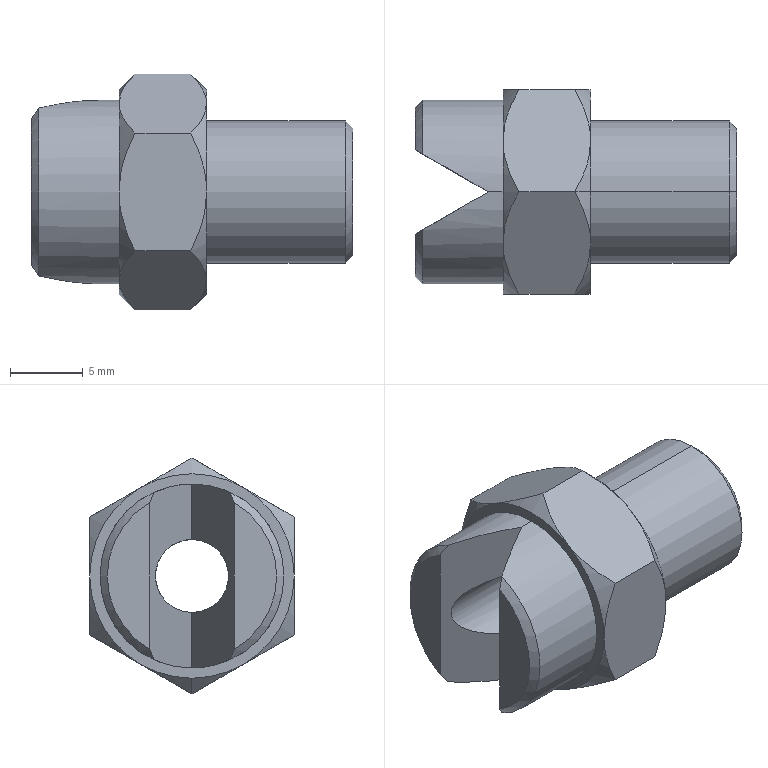Part | SolidWorks | features ICE 3, RevCut 1, Revolution 1 | 1 solid | 40 faces | box 22 x 14 x 16.166 mm | volume 1551 mm3 | cone 18 | plane 14 | cylinder 8 | commonest cylinder face diameters 5 x2 7.5 x2 9.728 x2 12.6 x2
STEP:
#1=CARTESIAN_POINT('',(5.,0.,2.5));
#2=VERTEX_POINT('',#1);
#3=CARTESIAN_POINT('',(5.,0.,-2.5));
#4=VERTEX_POINT('',#3);
#5=CARTESIAN_POINT('',(5.,0.,2.5));
#6=CARTESIAN_POINT('',(-3.66,-5.,2.5));
#7=CARTESIAN_POINT('',(-3.66,-5.,-2.5));
#8=CARTESIAN_POINT('',(5.,0.,-2.5));
#9=(BOUNDED_CURVE()B_SPLINE_CURVE(3,(#5,#6,#7,#8),.UNSPECIFIED.,.F.,.T.)B_SPLINE_CURVE_WITH_KNOTS((4,4),(1.571,4.712),.UNSPECIFIED.)CURVE()GEOMETRIC_REPRESENTATION_ITEM()RATIONAL_B_SPLINE_CURVE((1.,0.3333,0.3333,1.))REPRESENTATION_ITEM(''));
#10=EDGE_CURVE('',#2,#4,#9,.T.);
#11=ORIENTED_EDGE('',*,*,#10,.F.);
#12=CARTESIAN_POINT('',(6.,0.,2.5));
#13=VERTEX_POINT('',#12);
#14=CARTESIAN_POINT('',(0.,0.,2.5));
#15=DIRECTION('',(1.,0.,0.));
#16=VECTOR('',#15,1000.);
#17=LINE('',#14,#16);
#18=EDGE_CURVE('',#2,#13,#17,.T.);
#19=ORIENTED_EDGE('',*,*,#18,.T.);
#20=CARTESIAN_POINT('',(6.,0.,-2.5));
#21=VERTEX_POINT('',#20);
#22=CARTESIAN_POINT('',(6.,0.,0.));
#23=DIRECTION('',(1.,0.,0.));
#24=DIRECTION('',(0.,0.,-1.));
#25=AXIS2_PLACEMENT_3D('',#22,#23,#24);
#26=CIRCLE('',#25,2.5);
#27=EDGE_CURVE('',#13,#21,#26,.T.);
#28=ORIENTED_EDGE('',*,*,#27,.T.);
#29=CARTESIAN_POINT('',(0.,0.,-2.5));
#30=DIRECTION('',(1.,0.,0.));
#31=VECTOR('',#30,1000.);
#32=LINE('',#29,#31);
#33=EDGE_CURVE('',#4,#21,#32,.T.);
#34=ORIENTED_EDGE('',*,*,#33,.F.);
#35=EDGE_LOOP('',(#11,#19,#28,#34));
#36=FACE_OUTER_BOUND('',#35,.T.);
#37=CARTESIAN_POINT('',(0.,0.,0.));
#38=DIRECTION('',(1.,0.,0.));
#39=DIRECTION('',(0.,0.,-1.));
#40=AXIS2_PLACEMENT_3D('',#37,#38,#39);
#41=CYLINDRICAL_SURFACE('',#40,2.5);
#42=ADVANCED_FACE('',(#36),#41,.F.);
#43=CARTESIAN_POINT('',(6.,0.,6.3));
#44=VERTEX_POINT('',#43);
#45=CARTESIAN_POINT('',(6.,0.,-6.3));
#46=VERTEX_POINT('',#45);
#47=CARTESIAN_POINT('',(6.,0.,0.));
#48=DIRECTION('',(-1.,0.,0.));
#49=DIRECTION('',(0.,0.,1.));
#50=AXIS2_PLACEMENT_3D('',#47,#48,#49);
#51=CIRCLE('',#50,6.3);
#52=EDGE_CURVE('',#44,#46,#51,.T.);
#53=ORIENTED_EDGE('',*,*,#52,.T.);
#54=CARTESIAN_POINT('',(5.,0.,-6.3));
#55=VERTEX_POINT('',#54);
#56=CARTESIAN_POINT('',(0.,0.,-6.3));
#57=DIRECTION('',(-1.,0.,0.));
#58=VECTOR('',#57,1000.);
#59=LINE('',#56,#58);
#60=EDGE_CURVE('',#46,#55,#59,.T.);
#61=ORIENTED_EDGE('',*,*,#60,.T.);
#62=CARTESIAN_POINT('',(0.5,2.598,-5.739));
#63=VERTEX_POINT('',#62);
#64=CARTESIAN_POINT('',(5.,0.,-6.3));
#65=CARTESIAN_POINT('',(3.442,0.8995,-6.3));
#66=CARTESIAN_POINT('',(1.919,1.779,-6.11));
#67=CARTESIAN_POINT('',(0.5,2.598,-5.739));
#68=(BOUNDED_CURVE()B_SPLINE_CURVE(3,(#64,#65,#66,#67),.UNSPECIFIED.,.F.,.T.)B_SPLINE_CURVE_WITH_KNOTS((4,4),(4.712,5.137),.UNSPECIFIED.)CURVE()GEOMETRIC_REPRESENTATION_ITEM()RATIONAL_B_SPLINE_CURVE((1.,0.985,0.985,1.))REPRESENTATION_ITEM(''));
#69=EDGE_CURVE('',#55,#63,#68,.T.);
#70=ORIENTED_EDGE('',*,*,#69,.T.);
#71=CARTESIAN_POINT('',(0.5,2.598,5.739));
#72=VERTEX_POINT('',#71);
#73=CARTESIAN_POINT('',(0.5,0.,0.));
#74=DIRECTION('',(-1.,0.,0.));
#75=DIRECTION('',(0.,0.,1.));
#76=AXIS2_PLACEMENT_3D('',#73,#74,#75);
#77=CIRCLE('',#76,6.3);
#78=EDGE_CURVE('',#72,#63,#77,.T.);
#79=ORIENTED_EDGE('',*,*,#78,.F.);
#80=CARTESIAN_POINT('',(5.,0.,6.3));
#81=VERTEX_POINT('',#80);
#82=CARTESIAN_POINT('',(0.5,2.598,5.739));
#83=CARTESIAN_POINT('',(1.919,1.779,6.11));
#84=CARTESIAN_POINT('',(3.442,0.8995,6.3));
#85=CARTESIAN_POINT('',(5.,0.,6.3));
#86=(BOUNDED_CURVE()B_SPLINE_CURVE(3,(#82,#83,#84,#85),.UNSPECIFIED.,.F.,.F.)B_SPLINE_CURVE_WITH_KNOTS((4,4),(1.146,1.571),.UNSPECIFIED.)CURVE()GEOMETRIC_REPRESENTATION_ITEM()RATIONAL_B_SPLINE_CURVE((1.,0.985,0.985,1.))REPRESENTATION_ITEM(''));
#87=EDGE_CURVE('',#72,#81,#86,.T.);
#88=ORIENTED_EDGE('',*,*,#87,.T.);
#89=CARTESIAN_POINT('',(0.,0.,6.3));
#90=DIRECTION('',(-1.,0.,0.));
#91=VECTOR('',#90,1000.);
#92=LINE('',#89,#91);
#93=EDGE_CURVE('',#44,#81,#92,.T.);
#94=ORIENTED_EDGE('',*,*,#93,.F.);
#95=EDGE_LOOP('',(#53,#61,#70,#79,#88,#94));
#96=FACE_OUTER_BOUND('',#95,.T.);
#97=CARTESIAN_POINT('',(0.,0.,0.));
#98=DIRECTION('',(-1.,0.,0.));
#99=DIRECTION('',(0.,0.,1.));
#100=AXIS2_PLACEMENT_3D('',#97,#98,#99);
#101=CYLINDRICAL_SURFACE('',#100,6.3);
#102=ADVANCED_FACE('',(#96),#101,.T.);
#103=CARTESIAN_POINT('',(6.,-3.5,-6.062));
#104=VERTEX_POINT('',#103);
#105=CARTESIAN_POINT('',(6.,0.,-7.));
#106=VERTEX_POINT('',#105);
#107=CARTESIAN_POINT('',(6.,0.,0.));
#108=DIRECTION('',(1.,0.,0.));
#109=DIRECTION('',(0.,0.,-1.));
#110=AXIS2_PLACEMENT_3D('',#107,#108,#109);
#111=CIRCLE('',#110,7.);
#112=EDGE_CURVE('',#104,#106,#111,.T.);
#113=ORIENTED_EDGE('',*,*,#112,.T.);
#114=CARTESIAN_POINT('',(7.083,0.,-8.083));
#115=VERTEX_POINT('',#114);
#116=CARTESIAN_POINT('',(6.,0.,-7.));
#117=DIRECTION('',(0.7071,0.,-0.7071));
#118=VECTOR('',#117,1000.);
#119=LINE('',#116,#118);
#120=EDGE_CURVE('',#106,#115,#119,.T.);
#121=ORIENTED_EDGE('',*,*,#120,.T.);
#122=CARTESIAN_POINT('',(7.083,0.,-8.083));
#123=CARTESIAN_POINT('',(6.766,-0.5488,-7.766));
#124=CARTESIAN_POINT('',(6.497,-1.11,-7.442));
#125=CARTESIAN_POINT('',(6.209,-1.982,-6.938));
#126=CARTESIAN_POINT('',(6.132,-2.278,-6.768));
#127=CARTESIAN_POINT('',(6.028,-2.882,-6.419));
#128=CARTESIAN_POINT('',(6.,-3.193,-6.239));
#129=CARTESIAN_POINT('',(6.,-3.5,-6.062));
#130=B_SPLINE_CURVE_WITH_KNOTS('',3,(#122,#123,#124,#125,#126,#127,#128,#129),.UNSPECIFIED.,.F.,.F.,(4,2,2,4),(0.000000254,0.002095,0.003142,0.00419),.UNSPECIFIED.);
#131=EDGE_CURVE('',#115,#104,#130,.T.);
#132=ORIENTED_EDGE('',*,*,#131,.T.);
#133=EDGE_LOOP('',(#113,#121,#132));
#134=FACE_OUTER_BOUND('',#133,.T.);
#135=CARTESIAN_POINT('',(6.,0.,0.));
#136=DIRECTION('',(1.,0.,0.));
#137=DIRECTION('',(0.,0.,-1.));
#138=AXIS2_PLACEMENT_3D('',#135,#136,#137);
#139=CONICAL_SURFACE('',#138,7.,0.7854);
#140=ADVANCED_FACE('',(#134),#139,.T.);
#141=CARTESIAN_POINT('',(12.,0.,7.));
#142=VERTEX_POINT('',#141);
#143=CARTESIAN_POINT('',(12.,-3.5,6.062));
#144=VERTEX_POINT('',#143);
#145=CARTESIAN_POINT('',(12.,0.,0.));
#146=DIRECTION('',(1.,0.,0.));
#147=DIRECTION('',(0.,0.,-1.));
#148=AXIS2_PLACEMENT_3D('',#145,#146,#147);
#149=CIRCLE('',#148,7.);
#150=EDGE_CURVE('',#142,#144,#149,.T.);
#151=ORIENTED_EDGE('',*,*,#150,.F.);
#152=CARTESIAN_POINT('',(10.917,0.,8.083));
#153=VERTEX_POINT('',#152);
#154=CARTESIAN_POINT('',(10.917,0.,8.083));
#155=DIRECTION('',(-0.7071,0.,0.7071));
#156=VECTOR('',#155,1000.);
#157=LINE('',#154,#156);
#158=EDGE_CURVE('',#142,#153,#157,.T.);
#159=ORIENTED_EDGE('',*,*,#158,.T.);
#160=CARTESIAN_POINT('',(10.917,0.,8.083));
#161=CARTESIAN_POINT('',(11.234,-0.5488,7.766));
#162=CARTESIAN_POINT('',(11.503,-1.11,7.442));
#163=CARTESIAN_POINT('',(11.791,-1.982,6.938));
#164=CARTESIAN_POINT('',(11.868,-2.278,6.768));
#165=CARTESIAN_POINT('',(11.972,-2.882,6.419));
#166=CARTESIAN_POINT('',(12.,-3.193,6.239));
#167=CARTESIAN_POINT('',(12.,-3.5,6.062));
#168=B_SPLINE_CURVE_WITH_KNOTS('',3,(#160,#161,#162,#163,#164,#165,#166,#167),.UNSPECIFIED.,.F.,.F.,(4,2,2,4),(0.000000254,0.002095,0.003142,0.00419),.UNSPECIFIED.);
#169=EDGE_CURVE('',#153,#144,#168,.T.);
#170=ORIENTED_EDGE('',*,*,#169,.T.);
#171=EDGE_LOOP('',(#151,#159,#170));
#172=FACE_OUTER_BOUND('',#171,.T.);
#173=CARTESIAN_POINT('',(10.917,0.,0.));
#174=DIRECTION('',(-1.,0.,0.));
#175=DIRECTION('',(0.,0.,1.));
#176=AXIS2_PLACEMENT_3D('',#173,#174,#175);
#177=CONICAL_SURFACE('',#176,8.083,0.7854);
#178=ADVANCED_FACE('',(#172),#177,.T.);
#179=CARTESIAN_POINT('',(22.,0.,-3.75));
#180=VERTEX_POINT('',#179);
#181=CARTESIAN_POINT('',(22.,0.,3.75));
#182=VERTEX_POINT('',#181);
#183=CARTESIAN_POINT('',(22.,0.,0.));
#184=DIRECTION('',(-1.,0.,0.));
#185=DIRECTION('',(0.,0.,1.));
#186=AXIS2_PLACEMENT_3D('',#183,#184,#185);
#187=CIRCLE('',#186,3.75);
#188=EDGE_CURVE('',#180,#182,#187,.T.);
#189=ORIENTED_EDGE('',*,*,#188,.F.);
#190=CARTESIAN_POINT('',(6.,0.,-3.75));
#191=VERTEX_POINT('',#190);
#192=CARTESIAN_POINT('',(0.,0.,-3.75));
#193=DIRECTION('',(-1.,0.,0.));
#194=VECTOR('',#193,1000.);
#195=LINE('',#192,#194);
#196=EDGE_CURVE('',#180,#191,#195,.T.);
#197=ORIENTED_EDGE('',*,*,#196,.T.);
#198=CARTESIAN_POINT('',(6.,0.,3.75));
#199=VERTEX_POINT('',#198);
#200=CARTESIAN_POINT('',(6.,0.,0.));
#201=DIRECTION('',(-1.,0.,0.));
#202=DIRECTION('',(0.,0.,1.));
#203=AXIS2_PLACEMENT_3D('',#200,#201,#202);
#204=CIRCLE('',#203,3.75);
#205=EDGE_CURVE('',#191,#199,#204,.T.);
#206=ORIENTED_EDGE('',*,*,#205,.T.);
#207=CARTESIAN_POINT('',(0.,0.,3.75));
#208=DIRECTION('',(-1.,0.,0.));
#209=VECTOR('',#208,1000.);
#210=LINE('',#207,#209);
#211=EDGE_CURVE('',#182,#199,#210,.T.);
#212=ORIENTED_EDGE('',*,*,#211,.F.);
#213=EDGE_LOOP('',(#189,#197,#206,#212));
#214=FACE_OUTER_BOUND('',#213,.T.);
#215=CARTESIAN_POINT('',(0.,0.,0.));
#216=DIRECTION('',(-1.,0.,0.));
#217=DIRECTION('',(0.,0.,1.));
#218=AXIS2_PLACEMENT_3D('',#215,#216,#217);
#219=CYLINDRICAL_SURFACE('',#218,3.75);
#220=ADVANCED_FACE('',(#214),#219,.F.);
#221=CARTESIAN_POINT('',(22.,0.,4.364));
#222=VERTEX_POINT('',#221);
#223=CARTESIAN_POINT('',(22.,0.,-4.364));
#224=VERTEX_POINT('',#223);
#225=CARTESIAN_POINT('',(22.,0.,0.));
#226=DIRECTION('',(-1.,0.,0.));
#227=DIRECTION('',(0.,0.,1.));
#228=AXIS2_PLACEMENT_3D('',#225,#226,#227);
#229=CIRCLE('',#228,4.364);
#230=EDGE_CURVE('',#222,#224,#229,.T.);
#231=ORIENTED_EDGE('',*,*,#230,.T.);
#232=CARTESIAN_POINT('',(21.5,0.,-4.864));
#233=VERTEX_POINT('',#232);
#234=CARTESIAN_POINT('',(22.,0.,-4.364));
#235=DIRECTION('',(-0.7071,0.,-0.7071));
#236=VECTOR('',#235,1000.);
#237=LINE('',#234,#236);
#238=EDGE_CURVE('',#224,#233,#237,.T.);
#239=ORIENTED_EDGE('',*,*,#238,.T.);
#240=CARTESIAN_POINT('',(21.5,0.,4.864));
#241=VERTEX_POINT('',#240);
#242=CARTESIAN_POINT('',(21.5,0.,0.));
#243=DIRECTION('',(-1.,0.,0.));
#244=DIRECTION('',(0.,0.,1.));
#245=AXIS2_PLACEMENT_3D('',#242,#243,#244);
#246=CIRCLE('',#245,4.864);
#247=EDGE_CURVE('',#241,#233,#246,.T.);
#248=ORIENTED_EDGE('',*,*,#247,.F.);
#249=CARTESIAN_POINT('',(22.,0.,4.364));
#250=DIRECTION('',(-0.7071,0.,0.7071));
#251=VECTOR('',#250,1000.);
#252=LINE('',#249,#251);
#253=EDGE_CURVE('',#222,#241,#252,.T.);
#254=ORIENTED_EDGE('',*,*,#253,.F.);
#255=EDGE_LOOP('',(#231,#239,#248,#254));
#256=FACE_OUTER_BOUND('',#255,.T.);
#257=CARTESIAN_POINT('',(22.,0.,0.));
#258=DIRECTION('',(-1.,0.,0.));
#259=DIRECTION('',(0.,0.,1.));
#260=AXIS2_PLACEMENT_3D('',#257,#258,#259);
#261=CONICAL_SURFACE('',#260,4.364,0.7854);
#262=ADVANCED_FACE('',(#256),#261,.T.);
#263=ORIENTED_EDGE('',*,*,#247,.T.);
#264=CARTESIAN_POINT('',(12.,0.,-4.864));
#265=VERTEX_POINT('',#264);
#266=CARTESIAN_POINT('',(0.,0.,-4.864));
#267=DIRECTION('',(-1.,0.,0.));
#268=VECTOR('',#267,1000.);
#269=LINE('',#266,#268);
#270=EDGE_CURVE('',#233,#265,#269,.T.);
#271=ORIENTED_EDGE('',*,*,#270,.T.);
#272=CARTESIAN_POINT('',(12.,0.,4.864));
#273=VERTEX_POINT('',#272);
#274=CARTESIAN_POINT('',(12.,0.,0.));
#275=DIRECTION('',(-1.,0.,0.));
#276=DIRECTION('',(0.,0.,1.));
#277=AXIS2_PLACEMENT_3D('',#274,#275,#276);
#278=CIRCLE('',#277,4.864);
#279=EDGE_CURVE('',#273,#265,#278,.T.);
#280=ORIENTED_EDGE('',*,*,#279,.F.);
#281=CARTESIAN_POINT('',(0.,0.,4.864));
#282=DIRECTION('',(-1.,0.,0.));
#283=VECTOR('',#282,1000.);
#284=LINE('',#281,#283);
#285=EDGE_CURVE('',#241,#273,#284,.T.);
#286=ORIENTED_EDGE('',*,*,#285,.F.);
#287=EDGE_LOOP('',(#263,#271,#280,#286));
#288=FACE_OUTER_BOUND('',#287,.T.);
#289=CARTESIAN_POINT('',(0.,0.,0.));
#290=DIRECTION('',(-1.,0.,0.));
#291=DIRECTION('',(0.,0.,1.));
#292=AXIS2_PLACEMENT_3D('',#289,#290,#291);
#293=CYLINDRICAL_SURFACE('',#292,4.864);
#294=ADVANCED_FACE('',(#288),#293,.T.);
#295=CARTESIAN_POINT('',(0.,2.887,5.031));
#296=VERTEX_POINT('',#295);
#297=CARTESIAN_POINT('',(0.,2.887,-5.031));
#298=VERTEX_POINT('',#297);
#299=CARTESIAN_POINT('',(0.,0.,0.));
#300=DIRECTION('',(-1.,0.,0.));
#301=DIRECTION('',(0.,0.,1.));
#302=AXIS2_PLACEMENT_3D('',#299,#300,#301);
#303=CIRCLE('',#302,5.8);
#304=EDGE_CURVE('',#296,#298,#303,.T.);
#305=ORIENTED_EDGE('',*,*,#304,.T.);
#306=CARTESIAN_POINT('',(0.,2.887,-8.083));
#307=DIRECTION('',(0.,0.,1.));
#308=VECTOR('',#307,1000.);
#309=LINE('',#306,#308);
#310=EDGE_CURVE('',#298,#296,#309,.T.);
#311=ORIENTED_EDGE('',*,*,#310,.T.);
#312=EDGE_LOOP('',(#305,#311));
#313=FACE_OUTER_BOUND('',#312,.T.);
#314=CARTESIAN_POINT('',(0.,0.,0.));
#315=DIRECTION('',(1.,0.,0.));
#316=DIRECTION('',(0.,0.,-1.));
#317=AXIS2_PLACEMENT_3D('',#314,#315,#316);
#318=PLANE('',#317);
#319=ADVANCED_FACE('',(#313),#318,.F.);
#320=ORIENTED_EDGE('',*,*,#78,.T.);
#321=CARTESIAN_POINT('',(0.5,2.598,-5.739));
#322=CARTESIAN_POINT('',(0.3291,2.697,-5.507));
#323=CARTESIAN_POINT('',(0.1621,2.793,-5.271));
#324=CARTESIAN_POINT('',(0.,2.887,-5.031));
#325=B_SPLINE_CURVE_WITH_KNOTS('',3,(#321,#322,#323,#324),.UNSPECIFIED.,.F.,.F.,(4,4),(0.000000357,0.0009145),.UNSPECIFIED.);
#326=EDGE_CURVE('',#63,#298,#325,.T.);
#327=ORIENTED_EDGE('',*,*,#326,.T.);
#328=ORIENTED_EDGE('',*,*,#304,.F.);
#329=CARTESIAN_POINT('',(0.,2.887,5.031));
#330=CARTESIAN_POINT('',(0.1621,2.793,5.271));
#331=CARTESIAN_POINT('',(0.3291,2.697,5.507));
#332=CARTESIAN_POINT('',(0.5,2.598,5.739));
#333=B_SPLINE_CURVE_WITH_KNOTS('',3,(#329,#330,#331,#332),.UNSPECIFIED.,.F.,.F.,(4,4),(0.000000376,0.0009145),.UNSPECIFIED.);
#334=EDGE_CURVE('',#296,#72,#333,.T.);
#335=ORIENTED_EDGE('',*,*,#334,.T.);
#336=EDGE_LOOP('',(#320,#327,#328,#335));
#337=FACE_OUTER_BOUND('',#336,.T.);
#338=CARTESIAN_POINT('',(0.5,0.,0.));
#339=DIRECTION('',(1.,0.,0.));
#340=DIRECTION('',(0.,0.,-1.));
#341=AXIS2_PLACEMENT_3D('',#338,#339,#340);
#342=CONICAL_SURFACE('',#341,6.3,0.7854);
#343=ADVANCED_FACE('',(#337),#342,.T.);
#344=CARTESIAN_POINT('',(12.,3.5,6.062));
#345=VERTEX_POINT('',#344);
#346=CARTESIAN_POINT('',(12.,0.,0.));
#347=DIRECTION('',(1.,0.,0.));
#348=DIRECTION('',(0.,0.,-1.));
#349=AXIS2_PLACEMENT_3D('',#346,#347,#348);
#350=CIRCLE('',#349,7.);
#351=EDGE_CURVE('',#345,#142,#350,.T.);
#352=ORIENTED_EDGE('',*,*,#351,.T.);
#353=ORIENTED_EDGE('',*,*,#150,.T.);
#354=CARTESIAN_POINT('',(12.,-7.,0.));
#355=VERTEX_POINT('',#354);
#356=CARTESIAN_POINT('',(12.,0.,0.));
#357=DIRECTION('',(1.,0.,0.));
#358=DIRECTION('',(0.,0.,-1.));
#359=AXIS2_PLACEMENT_3D('',#356,#357,#358);
#360=CIRCLE('',#359,7.);
#361=EDGE_CURVE('',#144,#355,#360,.T.);
#362=ORIENTED_EDGE('',*,*,#361,.T.);
#363=CARTESIAN_POINT('',(12.,-3.5,-6.062));
#364=VERTEX_POINT('',#363);
#365=CARTESIAN_POINT('',(12.,0.,0.));
#366=DIRECTION('',(1.,0.,0.));
#367=DIRECTION('',(0.,0.,-1.));
#368=AXIS2_PLACEMENT_3D('',#365,#366,#367);
#369=CIRCLE('',#368,7.);
#370=EDGE_CURVE('',#355,#364,#369,.T.);
#371=ORIENTED_EDGE('',*,*,#370,.T.);
#372=CARTESIAN_POINT('',(12.,3.5,-6.062));
#373=VERTEX_POINT('',#372);
#374=CARTESIAN_POINT('',(12.,0.,0.));
#375=DIRECTION('',(1.,0.,0.));
#376=DIRECTION('',(0.,0.,-1.));
#377=AXIS2_PLACEMENT_3D('',#374,#375,#376);
#378=CIRCLE('',#377,7.);
#379=EDGE_CURVE('',#364,#373,#378,.T.);
#380=ORIENTED_EDGE('',*,*,#379,.T.);
#381=CARTESIAN_POINT('',(12.,7.,0.));
#382=VERTEX_POINT('',#381);
#383=CARTESIAN_POINT('',(12.,0.,0.));
#384=DIRECTION('',(1.,0.,0.));
#385=DIRECTION('',(0.,0.,-1.));
#386=AXIS2_PLACEMENT_3D('',#383,#384,#385);
#387=CIRCLE('',#386,7.);
#388=EDGE_CURVE('',#373,#382,#387,.T.);
#389=ORIENTED_EDGE('',*,*,#388,.T.);
#390=CARTESIAN_POINT('',(12.,0.,0.));
#391=DIRECTION('',(1.,0.,0.));
#392=DIRECTION('',(0.,0.,-1.));
#393=AXIS2_PLACEMENT_3D('',#390,#391,#392);
#394=CIRCLE('',#393,7.);
#395=EDGE_CURVE('',#382,#345,#394,.T.);
#396=ORIENTED_EDGE('',*,*,#395,.T.);
#397=EDGE_LOOP('',(#352,#353,#362,#371,#380,#389,#396));
#398=FACE_OUTER_BOUND('',#397,.T.);
#399=ORIENTED_EDGE('',*,*,#279,.T.);
#400=CARTESIAN_POINT('',(12.,0.,0.));
#401=DIRECTION('',(-1.,0.,0.));
#402=DIRECTION('',(0.,0.,1.));
#403=AXIS2_PLACEMENT_3D('',#400,#401,#402);
#404=CIRCLE('',#403,4.864);
#405=EDGE_CURVE('',#265,#273,#404,.T.);
#406=ORIENTED_EDGE('',*,*,#405,.T.);
#407=EDGE_LOOP('',(#399,#406));
#408=FACE_BOUND('',#407,.T.);
#409=CARTESIAN_POINT('',(12.,7.,0.));
#410=DIRECTION('',(-1.,0.,0.));
#411=DIRECTION('',(0.,0.,1.));
#412=AXIS2_PLACEMENT_3D('',#409,#410,#411);
#413=PLANE('',#412);
#414=ADVANCED_FACE('',(#398,#408),#413,.F.);
#415=ORIENTED_EDGE('',*,*,#270,.F.);
#416=CARTESIAN_POINT('',(21.5,0.,0.));
#417=DIRECTION('',(-1.,0.,0.));
#418=DIRECTION('',(0.,0.,1.));
#419=AXIS2_PLACEMENT_3D('',#416,#417,#418);
#420=CIRCLE('',#419,4.864);
#421=EDGE_CURVE('',#233,#241,#420,.T.);
#422=ORIENTED_EDGE('',*,*,#421,.T.);
#423=ORIENTED_EDGE('',*,*,#285,.T.);
#424=ORIENTED_EDGE('',*,*,#405,.F.);
#425=EDGE_LOOP('',(#415,#422,#423,#424));
#426=FACE_OUTER_BOUND('',#425,.T.);
#427=CARTESIAN_POINT('',(0.,0.,0.));
#428=DIRECTION('',(-1.,0.,0.));
#429=DIRECTION('',(0.,0.,1.));
#430=AXIS2_PLACEMENT_3D('',#427,#428,#429);
#431=CYLINDRICAL_SURFACE('',#430,4.864);
#432=ADVANCED_FACE('',(#426),#431,.T.);
#433=ORIENTED_EDGE('',*,*,#238,.F.);
#434=CARTESIAN_POINT('',(22.,0.,0.));
#435=DIRECTION('',(-1.,0.,0.));
#436=DIRECTION('',(0.,0.,1.));
#437=AXIS2_PLACEMENT_3D('',#434,#435,#436);
#438=CIRCLE('',#437,4.364);
#439=EDGE_CURVE('',#224,#222,#438,.T.);
#440=ORIENTED_EDGE('',*,*,#439,.T.);
#441=ORIENTED_EDGE('',*,*,#253,.T.);
#442=ORIENTED_EDGE('',*,*,#421,.F.);
#443=EDGE_LOOP('',(#433,#440,#441,#442));
#444=FACE_OUTER_BOUND('',#443,.T.);
#445=CARTESIAN_POINT('',(22.,0.,0.));
#446=DIRECTION('',(-1.,0.,0.));
#447=DIRECTION('',(0.,0.,1.));
#448=AXIS2_PLACEMENT_3D('',#445,#446,#447);
#449=CONICAL_SURFACE('',#448,4.364,0.7854);
#450=ADVANCED_FACE('',(#444),#449,.T.);
#451=ORIENTED_EDGE('',*,*,#230,.F.);
#452=ORIENTED_EDGE('',*,*,#439,.F.);
#453=EDGE_LOOP('',(#451,#452));
#454=FACE_OUTER_BOUND('',#453,.T.);
#455=CARTESIAN_POINT('',(22.,0.,0.));
#456=DIRECTION('',(-1.,0.,0.));
#457=DIRECTION('',(0.,0.,1.));
#458=AXIS2_PLACEMENT_3D('',#455,#456,#457);
#459=CIRCLE('',#458,3.75);
#460=EDGE_CURVE('',#182,#180,#459,.T.);
#461=ORIENTED_EDGE('',*,*,#460,.T.);
#462=ORIENTED_EDGE('',*,*,#188,.T.);
#463=EDGE_LOOP('',(#461,#462));
#464=FACE_BOUND('',#463,.T.);
#465=CARTESIAN_POINT('',(22.,4.364,0.));
#466=DIRECTION('',(-1.,0.,0.));
#467=DIRECTION('',(0.,0.,1.));
#468=AXIS2_PLACEMENT_3D('',#465,#466,#467);
#469=PLANE('',#468);
#470=ADVANCED_FACE('',(#454,#464),#469,.F.);
#471=ORIENTED_EDGE('',*,*,#196,.F.);
#472=ORIENTED_EDGE('',*,*,#460,.F.);
#473=ORIENTED_EDGE('',*,*,#211,.T.);
#474=CARTESIAN_POINT('',(6.,0.,0.));
#475=DIRECTION('',(-1.,0.,0.));
#476=DIRECTION('',(0.,0.,1.));
#477=AXIS2_PLACEMENT_3D('',#474,#475,#476);
#478=CIRCLE('',#477,3.75);
#479=EDGE_CURVE('',#199,#191,#478,.T.);
#480=ORIENTED_EDGE('',*,*,#479,.T.);
#481=EDGE_LOOP('',(#471,#472,#473,#480));
#482=FACE_OUTER_BOUND('',#481,.T.);
#483=CARTESIAN_POINT('',(0.,0.,0.));
#484=DIRECTION('',(-1.,0.,0.));
#485=DIRECTION('',(0.,0.,1.));
#486=AXIS2_PLACEMENT_3D('',#483,#484,#485);
#487=CYLINDRICAL_SURFACE('',#486,3.75);
#488=ADVANCED_FACE('',(#482),#487,.F.);
#489=CARTESIAN_POINT('',(6.,0.,0.));
#490=DIRECTION('',(1.,0.,0.));
#491=DIRECTION('',(0.,0.,-1.));
#492=AXIS2_PLACEMENT_3D('',#489,#490,#491);
#493=CIRCLE('',#492,2.5);
#494=EDGE_CURVE('',#21,#13,#493,.T.);
#495=ORIENTED_EDGE('',*,*,#494,.F.);
#496=ORIENTED_EDGE('',*,*,#27,.F.);
#497=EDGE_LOOP('',(#495,#496));
#498=FACE_BOUND('',#497,.T.);
#499=ORIENTED_EDGE('',*,*,#479,.F.);
#500=ORIENTED_EDGE('',*,*,#205,.F.);
#501=EDGE_LOOP('',(#499,#500));
#502=FACE_OUTER_BOUND('',#501,.T.);
#503=CARTESIAN_POINT('',(6.,3.75,0.));
#504=DIRECTION('',(-1.,0.,0.));
#505=DIRECTION('',(0.,0.,1.));
#506=AXIS2_PLACEMENT_3D('',#503,#504,#505);
#507=PLANE('',#506);
#508=ADVANCED_FACE('',(#498,#502),#507,.F.);
#509=CARTESIAN_POINT('',(10.917,0.,-8.083));
#510=VERTEX_POINT('',#509);
#511=CARTESIAN_POINT('',(10.917,0.,-8.083));
#512=CARTESIAN_POINT('',(11.234,0.5488,-7.766));
#513=CARTESIAN_POINT('',(11.503,1.11,-7.442));
#514=CARTESIAN_POINT('',(11.791,1.982,-6.938));
#515=CARTESIAN_POINT('',(11.868,2.278,-6.768));
#516=CARTESIAN_POINT('',(11.972,2.882,-6.419));
#517=CARTESIAN_POINT('',(12.,3.193,-6.239));
#518=CARTESIAN_POINT('',(12.,3.5,-6.062));
#519=B_SPLINE_CURVE_WITH_KNOTS('',3,(#511,#512,#513,#514,#515,#516,#517,#518),.UNSPECIFIED.,.F.,.F.,(4,2,2,4),(0.000000254,0.002095,0.003142,0.00419),.UNSPECIFIED.);
#520=EDGE_CURVE('',#510,#373,#519,.T.);
#521=ORIENTED_EDGE('',*,*,#520,.T.);
#522=ORIENTED_EDGE('',*,*,#379,.F.);
#523=CARTESIAN_POINT('',(12.,-3.5,-6.062));
#524=CARTESIAN_POINT('',(12.,-2.891,-6.414));
#525=CARTESIAN_POINT('',(11.893,-2.293,-6.759));
#526=CARTESIAN_POINT('',(11.505,-1.112,-7.441));
#527=CARTESIAN_POINT('',(11.234,-0.5482,-7.766));
#528=CARTESIAN_POINT('',(10.917,0.,-8.083));
#529=B_SPLINE_CURVE_WITH_KNOTS('',3,(#523,#524,#525,#526,#527,#528),.UNSPECIFIED.,.F.,.F.,(4,2,4),(0.00419,0.00627,0.00835),.UNSPECIFIED.);
#530=EDGE_CURVE('',#364,#510,#529,.T.);
#531=ORIENTED_EDGE('',*,*,#530,.T.);
#532=EDGE_LOOP('',(#521,#522,#531));
#533=FACE_OUTER_BOUND('',#532,.T.);
#534=CARTESIAN_POINT('',(10.917,0.,0.));
#535=DIRECTION('',(-1.,0.,0.));
#536=DIRECTION('',(0.,0.,1.));
#537=AXIS2_PLACEMENT_3D('',#534,#535,#536);
#538=CONICAL_SURFACE('',#537,8.083,0.7854);
#539=ADVANCED_FACE('',(#533),#538,.T.);
#540=CARTESIAN_POINT('',(10.917,-7.,-4.041));
#541=VERTEX_POINT('',#540);
#542=CARTESIAN_POINT('',(12.,-7.,0.));
#543=CARTESIAN_POINT('',(12.,-7.,-0.355));
#544=CARTESIAN_POINT('',(11.973,-7.,-0.7091));
#545=CARTESIAN_POINT('',(11.869,-7.,-1.402));
#546=CARTESIAN_POINT('',(11.793,-7.,-1.744));
#547=CARTESIAN_POINT('',(11.601,-7.,-2.418));
#548=CARTESIAN_POINT('',(11.485,-7.,-2.752));
#549=CARTESIAN_POINT('',(11.22,-7.,-3.408));
#550=CARTESIAN_POINT('',(11.074,-7.,-3.728));
#551=CARTESIAN_POINT('',(10.917,-7.,-4.041));
#552=B_SPLINE_CURVE_WITH_KNOTS('',3,(#542,#543,#544,#545,#546,#547,#548,#549,#550,#551),.UNSPECIFIED.,.F.,.F.,(4,2,2,2,4),(0.008486,0.009532,0.01058,0.01163,0.01267),.UNSPECIFIED.);
#553=EDGE_CURVE('',#355,#541,#552,.T.);
#554=ORIENTED_EDGE('',*,*,#553,.T.);
#555=CARTESIAN_POINT('',(10.917,-7.,-4.041));
#556=CARTESIAN_POINT('',(11.234,-6.451,-4.358));
#557=CARTESIAN_POINT('',(11.503,-5.89,-4.682));
#558=CARTESIAN_POINT('',(11.791,-5.018,-5.186));
#559=CARTESIAN_POINT('',(11.868,-4.722,-5.357));
#560=CARTESIAN_POINT('',(11.972,-4.118,-5.706));
#561=CARTESIAN_POINT('',(12.,-3.807,-5.885));
#562=CARTESIAN_POINT('',(12.,-3.5,-6.062));
#563=B_SPLINE_CURVE_WITH_KNOTS('',3,(#555,#556,#557,#558,#559,#560,#561,#562),.UNSPECIFIED.,.F.,.F.,(4,2,2,4),(0.000000254,0.002095,0.003142,0.00419),.UNSPECIFIED.);
#564=EDGE_CURVE('',#541,#364,#563,.T.);
#565=ORIENTED_EDGE('',*,*,#564,.T.);
#566=ORIENTED_EDGE('',*,*,#370,.F.);
#567=EDGE_LOOP('',(#554,#565,#566));
#568=FACE_OUTER_BOUND('',#567,.T.);
#569=CARTESIAN_POINT('',(10.917,0.,0.));
#570=DIRECTION('',(-1.,0.,0.));
#571=DIRECTION('',(0.,0.,1.));
#572=AXIS2_PLACEMENT_3D('',#569,#570,#571);
#573=CONICAL_SURFACE('',#572,8.083,0.7854);
#574=ADVANCED_FACE('',(#568),#573,.T.);
#575=CARTESIAN_POINT('',(10.917,-7.,4.041));
#576=VERTEX_POINT('',#575);
#577=CARTESIAN_POINT('',(12.,-3.5,6.062));
#578=CARTESIAN_POINT('',(12.,-4.109,5.711));
#579=CARTESIAN_POINT('',(11.893,-4.707,5.365));
#580=CARTESIAN_POINT('',(11.505,-5.888,4.684));
#581=CARTESIAN_POINT('',(11.234,-6.452,4.358));
#582=CARTESIAN_POINT('',(10.917,-7.,4.041));
#583=B_SPLINE_CURVE_WITH_KNOTS('',3,(#577,#578,#579,#580,#581,#582),.UNSPECIFIED.,.F.,.F.,(4,2,4),(0.00419,0.00627,0.00835),.UNSPECIFIED.);
#584=EDGE_CURVE('',#144,#576,#583,.T.);
#585=ORIENTED_EDGE('',*,*,#584,.T.);
#586=CARTESIAN_POINT('',(10.917,-7.,4.041));
#587=CARTESIAN_POINT('',(11.073,-7.,3.729));
#588=CARTESIAN_POINT('',(11.219,-7.,3.41));
#589=CARTESIAN_POINT('',(11.483,-7.,2.756));
#590=CARTESIAN_POINT('',(11.601,-7.,2.419));
#591=CARTESIAN_POINT('',(11.89,-7.,1.403));
#592=CARTESIAN_POINT('',(12.,-7.,0.7107));
#593=CARTESIAN_POINT('',(12.,-7.,0.));
#594=B_SPLINE_CURVE_WITH_KNOTS('',3,(#586,#587,#588,#589,#590,#591,#592,#593),.UNSPECIFIED.,.F.,.F.,(4,2,2,4),(0.004297,0.005344,0.006392,0.008486),.UNSPECIFIED.);
#595=EDGE_CURVE('',#576,#355,#594,.T.);
#596=ORIENTED_EDGE('',*,*,#595,.T.);
#597=ORIENTED_EDGE('',*,*,#361,.F.);
#598=EDGE_LOOP('',(#585,#596,#597));
#599=FACE_OUTER_BOUND('',#598,.T.);
#600=CARTESIAN_POINT('',(10.917,0.,0.));
#601=DIRECTION('',(-1.,0.,0.));
#602=DIRECTION('',(0.,0.,1.));
#603=AXIS2_PLACEMENT_3D('',#600,#601,#602);
#604=CONICAL_SURFACE('',#603,8.083,0.7854);
#605=ADVANCED_FACE('',(#599),#604,.T.);
#606=ORIENTED_EDGE('',*,*,#158,.F.);
#607=ORIENTED_EDGE('',*,*,#351,.F.);
#608=CARTESIAN_POINT('',(12.,3.5,6.062));
#609=CARTESIAN_POINT('',(12.,2.891,6.414));
#610=CARTESIAN_POINT('',(11.893,2.293,6.759));
#611=CARTESIAN_POINT('',(11.505,1.112,7.441));
#612=CARTESIAN_POINT('',(11.234,0.5482,7.766));
#613=CARTESIAN_POINT('',(10.917,0.,8.083));
#614=B_SPLINE_CURVE_WITH_KNOTS('',3,(#608,#609,#610,#611,#612,#613),.UNSPECIFIED.,.F.,.F.,(4,2,4),(0.00419,0.00627,0.00835),.UNSPECIFIED.);
#615=EDGE_CURVE('',#345,#153,#614,.T.);
#616=ORIENTED_EDGE('',*,*,#615,.T.);
#617=EDGE_LOOP('',(#606,#607,#616));
#618=FACE_OUTER_BOUND('',#617,.T.);
#619=CARTESIAN_POINT('',(10.917,0.,0.));
#620=DIRECTION('',(-1.,0.,0.));
#621=DIRECTION('',(0.,0.,1.));
#622=AXIS2_PLACEMENT_3D('',#619,#620,#621);
#623=CONICAL_SURFACE('',#622,8.083,0.7854);
#624=ADVANCED_FACE('',(#618),#623,.T.);
#625=CARTESIAN_POINT('',(10.917,7.,4.041));
#626=VERTEX_POINT('',#625);
#627=CARTESIAN_POINT('',(12.,7.,0.));
#628=CARTESIAN_POINT('',(12.,7.,0.7107));
#629=CARTESIAN_POINT('',(11.89,7.,1.403));
#630=CARTESIAN_POINT('',(11.601,7.,2.419));
#631=CARTESIAN_POINT('',(11.483,7.,2.756));
#632=CARTESIAN_POINT('',(11.219,7.,3.41));
#633=CARTESIAN_POINT('',(11.073,7.,3.729));
#634=CARTESIAN_POINT('',(10.917,7.,4.041));
#635=B_SPLINE_CURVE_WITH_KNOTS('',3,(#627,#628,#629,#630,#631,#632,#633,#634),.UNSPECIFIED.,.F.,.F.,(4,2,2,4),(0.009437,0.01153,0.01258,0.01363),.UNSPECIFIED.);
#636=EDGE_CURVE('',#382,#626,#635,.T.);
#637=ORIENTED_EDGE('',*,*,#636,.T.);
#638=CARTESIAN_POINT('',(10.917,7.,4.041));
#639=CARTESIAN_POINT('',(11.234,6.451,4.358));
#640=CARTESIAN_POINT('',(11.503,5.89,4.682));
#641=CARTESIAN_POINT('',(11.791,5.018,5.186));
#642=CARTESIAN_POINT('',(11.868,4.722,5.357));
#643=CARTESIAN_POINT('',(11.972,4.118,5.706));
#644=CARTESIAN_POINT('',(12.,3.807,5.885));
#645=CARTESIAN_POINT('',(12.,3.5,6.062));
#646=B_SPLINE_CURVE_WITH_KNOTS('',3,(#638,#639,#640,#641,#642,#643,#644,#645),.UNSPECIFIED.,.F.,.F.,(4,2,2,4),(0.000000254,0.002095,0.003142,0.00419),.UNSPECIFIED.);
#647=EDGE_CURVE('',#626,#345,#646,.T.);
#648=ORIENTED_EDGE('',*,*,#647,.T.);
#649=ORIENTED_EDGE('',*,*,#395,.F.);
#650=EDGE_LOOP('',(#637,#648,#649));
#651=FACE_OUTER_BOUND('',#650,.T.);
#652=CARTESIAN_POINT('',(10.917,0.,0.));
#653=DIRECTION('',(-1.,0.,0.));
#654=DIRECTION('',(0.,0.,1.));
#655=AXIS2_PLACEMENT_3D('',#652,#653,#654);
#656=CONICAL_SURFACE('',#655,8.083,0.7854);
#657=ADVANCED_FACE('',(#651),#656,.T.);
#658=CARTESIAN_POINT('',(10.917,7.,-4.041));
#659=VERTEX_POINT('',#658);
#660=CARTESIAN_POINT('',(12.,3.5,-6.062));
#661=CARTESIAN_POINT('',(12.,4.109,-5.711));
#662=CARTESIAN_POINT('',(11.893,4.707,-5.365));
#663=CARTESIAN_POINT('',(11.505,5.888,-4.684));
#664=CARTESIAN_POINT('',(11.234,6.452,-4.358));
#665=CARTESIAN_POINT('',(10.917,7.,-4.041));
#666=B_SPLINE_CURVE_WITH_KNOTS('',3,(#660,#661,#662,#663,#664,#665),.UNSPECIFIED.,.F.,.F.,(4,2,4),(0.00419,0.00627,0.00835),.UNSPECIFIED.);
#667=EDGE_CURVE('',#373,#659,#666,.T.);
#668=ORIENTED_EDGE('',*,*,#667,.T.);
#669=CARTESIAN_POINT('',(10.917,7.,-4.041));
#670=CARTESIAN_POINT('',(11.074,7.,-3.728));
#671=CARTESIAN_POINT('',(11.22,7.,-3.408));
#672=CARTESIAN_POINT('',(11.485,7.,-2.752));
#673=CARTESIAN_POINT('',(11.601,7.,-2.418));
#674=CARTESIAN_POINT('',(11.793,7.,-1.744));
#675=CARTESIAN_POINT('',(11.869,7.,-1.402));
#676=CARTESIAN_POINT('',(11.973,7.,-0.7091));
#677=CARTESIAN_POINT('',(12.,7.,-0.355));
#678=CARTESIAN_POINT('',(12.,7.,0.));
#679=B_SPLINE_CURVE_WITH_KNOTS('',3,(#669,#670,#671,#672,#673,#674,#675,#676,#677,#678),.UNSPECIFIED.,.F.,.F.,(4,2,2,2,4),(0.005249,0.006296,0.007343,0.00839,0.009437),.UNSPECIFIED.);
#680=EDGE_CURVE('',#659,#382,#679,.T.);
#681=ORIENTED_EDGE('',*,*,#680,.T.);
#682=ORIENTED_EDGE('',*,*,#388,.F.);
#683=EDGE_LOOP('',(#668,#681,#682));
#684=FACE_OUTER_BOUND('',#683,.T.);
#685=CARTESIAN_POINT('',(10.917,0.,0.));
#686=DIRECTION('',(-1.,0.,0.));
#687=DIRECTION('',(0.,0.,1.));
#688=AXIS2_PLACEMENT_3D('',#685,#686,#687);
#689=CONICAL_SURFACE('',#688,8.083,0.7854);
#690=ADVANCED_FACE('',(#684),#689,.T.);
#691=ORIENTED_EDGE('',*,*,#131,.F.);
#692=CARTESIAN_POINT('',(-15.385,0.,-8.083));
#693=DIRECTION('',(1.,0.,0.));
#694=VECTOR('',#693,1000.);
#695=LINE('',#692,#694);
#696=EDGE_CURVE('',#115,#510,#695,.T.);
#697=ORIENTED_EDGE('',*,*,#696,.T.);
#698=ORIENTED_EDGE('',*,*,#530,.F.);
#699=ORIENTED_EDGE('',*,*,#564,.F.);
#700=CARTESIAN_POINT('',(7.083,-7.,-4.041));
#701=VERTEX_POINT('',#700);
#702=CARTESIAN_POINT('',(-15.385,-7.,-4.041));
#703=DIRECTION('',(1.,0.,0.));
#704=VECTOR('',#703,1000.);
#705=LINE('',#702,#704);
#706=EDGE_CURVE('',#701,#541,#705,.T.);
#707=ORIENTED_EDGE('',*,*,#706,.F.);
#708=CARTESIAN_POINT('',(6.,-3.5,-6.062));
#709=CARTESIAN_POINT('',(6.,-4.109,-5.711));
#710=CARTESIAN_POINT('',(6.107,-4.707,-5.365));
#711=CARTESIAN_POINT('',(6.495,-5.888,-4.684));
#712=CARTESIAN_POINT('',(6.766,-6.452,-4.358));
#713=CARTESIAN_POINT('',(7.083,-7.,-4.041));
#714=B_SPLINE_CURVE_WITH_KNOTS('',3,(#708,#709,#710,#711,#712,#713),.UNSPECIFIED.,.F.,.F.,(4,2,4),(0.00419,0.00627,0.00835),.UNSPECIFIED.);
#715=EDGE_CURVE('',#104,#701,#714,.T.);
#716=ORIENTED_EDGE('',*,*,#715,.F.);
#717=EDGE_LOOP('',(#691,#697,#698,#699,#707,#716));
#718=FACE_OUTER_BOUND('',#717,.T.);
#719=CARTESIAN_POINT('',(-15.385,-7.,-4.041));
#720=DIRECTION('',(0.,-0.5,-0.866));
#721=DIRECTION('',(0.,0.866,-0.5));
#722=AXIS2_PLACEMENT_3D('',#719,#720,#721);
#723=PLANE('',#722);
#724=ADVANCED_FACE('',(#718),#723,.T.);
#725=CARTESIAN_POINT('',(6.,-7.,0.));
#726=VERTEX_POINT('',#725);
#727=CARTESIAN_POINT('',(7.083,-7.,-4.041));
#728=CARTESIAN_POINT('',(6.926,-7.,-3.728));
#729=CARTESIAN_POINT('',(6.78,-7.,-3.408));
#730=CARTESIAN_POINT('',(6.515,-7.,-2.752));
#731=CARTESIAN_POINT('',(6.399,-7.,-2.418));
#732=CARTESIAN_POINT('',(6.207,-7.,-1.744));
#733=CARTESIAN_POINT('',(6.131,-7.,-1.402));
#734=CARTESIAN_POINT('',(6.027,-7.,-0.7091));
#735=CARTESIAN_POINT('',(6.,-7.,-0.355));
#736=CARTESIAN_POINT('',(6.,-7.,0.));
#737=B_SPLINE_CURVE_WITH_KNOTS('',3,(#727,#728,#729,#730,#731,#732,#733,#734,#735,#736),.UNSPECIFIED.,.F.,.F.,(4,2,2,2,4),(0.005249,0.006296,0.007343,0.00839,0.009437),.UNSPECIFIED.);
#738=EDGE_CURVE('',#701,#726,#737,.T.);
#739=ORIENTED_EDGE('',*,*,#738,.F.);
#740=ORIENTED_EDGE('',*,*,#706,.T.);
#741=ORIENTED_EDGE('',*,*,#553,.F.);
#742=ORIENTED_EDGE('',*,*,#595,.F.);
#743=CARTESIAN_POINT('',(7.083,-7.,4.041));
#744=VERTEX_POINT('',#743);
#745=CARTESIAN_POINT('',(-15.385,-7.,4.041));
#746=DIRECTION('',(1.,0.,0.));
#747=VECTOR('',#746,1000.);
#748=LINE('',#745,#747);
#749=EDGE_CURVE('',#744,#576,#748,.T.);
#750=ORIENTED_EDGE('',*,*,#749,.F.);
#751=CARTESIAN_POINT('',(6.,-7.,0.));
#752=CARTESIAN_POINT('',(6.,-7.,0.7107));
#753=CARTESIAN_POINT('',(6.11,-7.,1.403));
#754=CARTESIAN_POINT('',(6.399,-7.,2.419));
#755=CARTESIAN_POINT('',(6.517,-7.,2.756));
#756=CARTESIAN_POINT('',(6.781,-7.,3.41));
#757=CARTESIAN_POINT('',(6.927,-7.,3.729));
#758=CARTESIAN_POINT('',(7.083,-7.,4.041));
#759=B_SPLINE_CURVE_WITH_KNOTS('',3,(#751,#752,#753,#754,#755,#756,#757,#758),.UNSPECIFIED.,.F.,.F.,(4,2,2,4),(0.009437,0.01153,0.01258,0.01363),.UNSPECIFIED.);
#760=EDGE_CURVE('',#726,#744,#759,.T.);
#761=ORIENTED_EDGE('',*,*,#760,.F.);
#762=EDGE_LOOP('',(#739,#740,#741,#742,#750,#761));
#763=FACE_OUTER_BOUND('',#762,.T.);
#764=CARTESIAN_POINT('',(-15.385,-7.,4.041));
#765=DIRECTION('',(0.,-1.,0.));
#766=DIRECTION('',(0.,0.,-1.));
#767=AXIS2_PLACEMENT_3D('',#764,#765,#766);
#768=PLANE('',#767);
#769=ADVANCED_FACE('',(#763),#768,.T.);
#770=CARTESIAN_POINT('',(6.,-3.5,6.062));
#771=VERTEX_POINT('',#770);
#772=CARTESIAN_POINT('',(7.083,-7.,4.041));
#773=CARTESIAN_POINT('',(6.766,-6.451,4.358));
#774=CARTESIAN_POINT('',(6.497,-5.89,4.682));
#775=CARTESIAN_POINT('',(6.209,-5.018,5.186));
#776=CARTESIAN_POINT('',(6.132,-4.722,5.357));
#777=CARTESIAN_POINT('',(6.028,-4.118,5.706));
#778=CARTESIAN_POINT('',(6.,-3.807,5.885));
#779=CARTESIAN_POINT('',(6.,-3.5,6.062));
#780=B_SPLINE_CURVE_WITH_KNOTS('',3,(#772,#773,#774,#775,#776,#777,#778,#779),.UNSPECIFIED.,.F.,.F.,(4,2,2,4),(0.000000254,0.002095,0.003142,0.00419),.UNSPECIFIED.);
#781=EDGE_CURVE('',#744,#771,#780,.T.);
#782=ORIENTED_EDGE('',*,*,#781,.F.);
#783=ORIENTED_EDGE('',*,*,#749,.T.);
#784=ORIENTED_EDGE('',*,*,#584,.F.);
#785=ORIENTED_EDGE('',*,*,#169,.F.);
#786=CARTESIAN_POINT('',(7.083,0.,8.083));
#787=VERTEX_POINT('',#786);
#788=CARTESIAN_POINT('',(-15.385,0.,8.083));
#789=DIRECTION('',(1.,0.,0.));
#790=VECTOR('',#789,1000.);
#791=LINE('',#788,#790);
#792=EDGE_CURVE('',#787,#153,#791,.T.);
#793=ORIENTED_EDGE('',*,*,#792,.F.);
#794=CARTESIAN_POINT('',(6.,-3.5,6.062));
#795=CARTESIAN_POINT('',(6.,-2.891,6.414));
#796=CARTESIAN_POINT('',(6.107,-2.293,6.759));
#797=CARTESIAN_POINT('',(6.495,-1.112,7.441));
#798=CARTESIAN_POINT('',(6.766,-0.5482,7.766));
#799=CARTESIAN_POINT('',(7.083,0.,8.083));
#800=B_SPLINE_CURVE_WITH_KNOTS('',3,(#794,#795,#796,#797,#798,#799),.UNSPECIFIED.,.F.,.F.,(4,2,4),(0.00419,0.00627,0.00835),.UNSPECIFIED.);
#801=EDGE_CURVE('',#771,#787,#800,.T.);
#802=ORIENTED_EDGE('',*,*,#801,.F.);
#803=EDGE_LOOP('',(#782,#783,#784,#785,#793,#802));
#804=FACE_OUTER_BOUND('',#803,.T.);
#805=CARTESIAN_POINT('',(-15.385,0.,8.083));
#806=DIRECTION('',(0.,-0.5,0.866));
#807=DIRECTION('',(0.,-0.866,-0.5));
#808=AXIS2_PLACEMENT_3D('',#805,#806,#807);
#809=PLANE('',#808);
#810=ADVANCED_FACE('',(#804),#809,.T.);
#811=CARTESIAN_POINT('',(6.,3.5,6.062));
#812=VERTEX_POINT('',#811);
#813=CARTESIAN_POINT('',(7.083,0.,8.083));
#814=CARTESIAN_POINT('',(6.766,0.5488,7.766));
#815=CARTESIAN_POINT('',(6.497,1.11,7.442));
#816=CARTESIAN_POINT('',(6.209,1.982,6.938));
#817=CARTESIAN_POINT('',(6.132,2.278,6.768));
#818=CARTESIAN_POINT('',(6.028,2.882,6.419));
#819=CARTESIAN_POINT('',(6.,3.193,6.239));
#820=CARTESIAN_POINT('',(6.,3.5,6.062));
#821=B_SPLINE_CURVE_WITH_KNOTS('',3,(#813,#814,#815,#816,#817,#818,#819,#820),.UNSPECIFIED.,.F.,.F.,(4,2,2,4),(0.000000254,0.002095,0.003142,0.00419),.UNSPECIFIED.);
#822=EDGE_CURVE('',#787,#812,#821,.T.);
#823=ORIENTED_EDGE('',*,*,#822,.F.);
#824=ORIENTED_EDGE('',*,*,#792,.T.);
#825=ORIENTED_EDGE('',*,*,#615,.F.);
#826=ORIENTED_EDGE('',*,*,#647,.F.);
#827=CARTESIAN_POINT('',(7.083,7.,4.041));
#828=VERTEX_POINT('',#827);
#829=CARTESIAN_POINT('',(-15.385,7.,4.041));
#830=DIRECTION('',(1.,0.,0.));
#831=VECTOR('',#830,1000.);
#832=LINE('',#829,#831);
#833=EDGE_CURVE('',#828,#626,#832,.T.);
#834=ORIENTED_EDGE('',*,*,#833,.F.);
#835=CARTESIAN_POINT('',(6.,3.5,6.062));
#836=CARTESIAN_POINT('',(6.,4.109,5.711));
#837=CARTESIAN_POINT('',(6.107,4.707,5.365));
#838=CARTESIAN_POINT('',(6.495,5.888,4.684));
#839=CARTESIAN_POINT('',(6.766,6.452,4.358));
#840=CARTESIAN_POINT('',(7.083,7.,4.041));
#841=B_SPLINE_CURVE_WITH_KNOTS('',3,(#835,#836,#837,#838,#839,#840),.UNSPECIFIED.,.F.,.F.,(4,2,4),(0.00419,0.00627,0.00835),.UNSPECIFIED.);
#842=EDGE_CURVE('',#812,#828,#841,.T.);
#843=ORIENTED_EDGE('',*,*,#842,.F.);
#844=EDGE_LOOP('',(#823,#824,#825,#826,#834,#843));
#845=FACE_OUTER_BOUND('',#844,.T.);
#846=CARTESIAN_POINT('',(-15.385,7.,4.041));
#847=DIRECTION('',(0.,0.5,0.866));
#848=DIRECTION('',(0.,-0.866,0.5));
#849=AXIS2_PLACEMENT_3D('',#846,#847,#848);
#850=PLANE('',#849);
#851=ADVANCED_FACE('',(#845),#850,.T.);
#852=CARTESIAN_POINT('',(6.,7.,0.));
#853=VERTEX_POINT('',#852);
#854=CARTESIAN_POINT('',(7.083,7.,4.041));
#855=CARTESIAN_POINT('',(6.927,7.,3.729));
#856=CARTESIAN_POINT('',(6.781,7.,3.41));
#857=CARTESIAN_POINT('',(6.517,7.,2.756));
#858=CARTESIAN_POINT('',(6.399,7.,2.419));
#859=CARTESIAN_POINT('',(6.11,7.,1.403));
#860=CARTESIAN_POINT('',(6.,7.,0.7107));
#861=CARTESIAN_POINT('',(6.,7.,0.));
#862=B_SPLINE_CURVE_WITH_KNOTS('',3,(#854,#855,#856,#857,#858,#859,#860,#861),.UNSPECIFIED.,.F.,.F.,(4,2,2,4),(0.004297,0.005344,0.006392,0.008486),.UNSPECIFIED.);
#863=EDGE_CURVE('',#828,#853,#862,.T.);
#864=ORIENTED_EDGE('',*,*,#863,.F.);
#865=ORIENTED_EDGE('',*,*,#833,.T.);
#866=ORIENTED_EDGE('',*,*,#636,.F.);
#867=ORIENTED_EDGE('',*,*,#680,.F.);
#868=CARTESIAN_POINT('',(7.083,7.,-4.041));
#869=VERTEX_POINT('',#868);
#870=CARTESIAN_POINT('',(-15.385,7.,-4.041));
#871=DIRECTION('',(1.,0.,0.));
#872=VECTOR('',#871,1000.);
#873=LINE('',#870,#872);
#874=EDGE_CURVE('',#869,#659,#873,.T.);
#875=ORIENTED_EDGE('',*,*,#874,.F.);
#876=CARTESIAN_POINT('',(6.,7.,0.));
#877=CARTESIAN_POINT('',(6.,7.,-0.355));
#878=CARTESIAN_POINT('',(6.027,7.,-0.7091));
#879=CARTESIAN_POINT('',(6.131,7.,-1.402));
#880=CARTESIAN_POINT('',(6.207,7.,-1.744));
#881=CARTESIAN_POINT('',(6.399,7.,-2.418));
#882=CARTESIAN_POINT('',(6.515,7.,-2.752));
#883=CARTESIAN_POINT('',(6.78,7.,-3.408));
#884=CARTESIAN_POINT('',(6.926,7.,-3.728));
#885=CARTESIAN_POINT('',(7.083,7.,-4.041));
#886=B_SPLINE_CURVE_WITH_KNOTS('',3,(#876,#877,#878,#879,#880,#881,#882,#883,#884,#885),.UNSPECIFIED.,.F.,.F.,(4,2,2,2,4),(0.008486,0.009532,0.01058,0.01163,0.01267),.UNSPECIFIED.);
#887=EDGE_CURVE('',#853,#869,#886,.T.);
#888=ORIENTED_EDGE('',*,*,#887,.F.);
#889=EDGE_LOOP('',(#864,#865,#866,#867,#875,#888));
#890=FACE_OUTER_BOUND('',#889,.T.);
#891=CARTESIAN_POINT('',(-15.385,7.,-4.041));
#892=DIRECTION('',(0.,1.,0.));
#893=DIRECTION('',(0.,0.,1.));
#894=AXIS2_PLACEMENT_3D('',#891,#892,#893);
#895=PLANE('',#894);
#896=ADVANCED_FACE('',(#890),#895,.T.);
#897=CARTESIAN_POINT('',(6.,3.5,-6.062));
#898=VERTEX_POINT('',#897);
#899=CARTESIAN_POINT('',(7.083,7.,-4.041));
#900=CARTESIAN_POINT('',(6.766,6.451,-4.358));
#901=CARTESIAN_POINT('',(6.497,5.89,-4.682));
#902=CARTESIAN_POINT('',(6.209,5.018,-5.186));
#903=CARTESIAN_POINT('',(6.132,4.722,-5.357));
#904=CARTESIAN_POINT('',(6.028,4.118,-5.706));
#905=CARTESIAN_POINT('',(6.,3.807,-5.885));
#906=CARTESIAN_POINT('',(6.,3.5,-6.062));
#907=B_SPLINE_CURVE_WITH_KNOTS('',3,(#899,#900,#901,#902,#903,#904,#905,#906),.UNSPECIFIED.,.F.,.F.,(4,2,2,4),(0.000000254,0.002095,0.003142,0.00419),.UNSPECIFIED.);
#908=EDGE_CURVE('',#869,#898,#907,.T.);
#909=ORIENTED_EDGE('',*,*,#908,.F.);
#910=ORIENTED_EDGE('',*,*,#874,.T.);
#911=ORIENTED_EDGE('',*,*,#667,.F.);
#912=ORIENTED_EDGE('',*,*,#520,.F.);
#913=ORIENTED_EDGE('',*,*,#696,.F.);
#914=CARTESIAN_POINT('',(6.,3.5,-6.062));
#915=CARTESIAN_POINT('',(6.,2.891,-6.414));
#916=CARTESIAN_POINT('',(6.107,2.293,-6.759));
#917=CARTESIAN_POINT('',(6.495,1.112,-7.441));
#918=CARTESIAN_POINT('',(6.766,0.5482,-7.766));
#919=CARTESIAN_POINT('',(7.083,0.,-8.083));
#920=B_SPLINE_CURVE_WITH_KNOTS('',3,(#914,#915,#916,#917,#918,#919),.UNSPECIFIED.,.F.,.F.,(4,2,4),(0.00419,0.00627,0.00835),.UNSPECIFIED.);
#921=EDGE_CURVE('',#898,#115,#920,.T.);
#922=ORIENTED_EDGE('',*,*,#921,.F.);
#923=EDGE_LOOP('',(#909,#910,#911,#912,#913,#922));
#924=FACE_OUTER_BOUND('',#923,.T.);
#925=CARTESIAN_POINT('',(-15.385,0.,-8.083));
#926=DIRECTION('',(0.,0.5,-0.866));
#927=DIRECTION('',(0.,0.866,0.5));
#928=AXIS2_PLACEMENT_3D('',#925,#926,#927);
#929=PLANE('',#928);
#930=ADVANCED_FACE('',(#924),#929,.T.);
#931=ORIENTED_EDGE('',*,*,#120,.F.);
#932=CARTESIAN_POINT('',(6.,0.,0.));
#933=DIRECTION('',(1.,0.,0.));
#934=DIRECTION('',(0.,0.,-1.));
#935=AXIS2_PLACEMENT_3D('',#932,#933,#934);
#936=CIRCLE('',#935,7.);
#937=EDGE_CURVE('',#106,#898,#936,.T.);
#938=ORIENTED_EDGE('',*,*,#937,.T.);
#939=ORIENTED_EDGE('',*,*,#921,.T.);
#940=EDGE_LOOP('',(#931,#938,#939));
#941=FACE_OUTER_BOUND('',#940,.T.);
#942=CARTESIAN_POINT('',(6.,0.,0.));
#943=DIRECTION('',(1.,0.,0.));
#944=DIRECTION('',(0.,0.,-1.));
#945=AXIS2_PLACEMENT_3D('',#942,#943,#944);
#946=CONICAL_SURFACE('',#945,7.,0.7854);
#947=ADVANCED_FACE('',(#941),#946,.T.);
#948=ORIENTED_EDGE('',*,*,#887,.T.);
#949=ORIENTED_EDGE('',*,*,#908,.T.);
#950=CARTESIAN_POINT('',(6.,0.,0.));
#951=DIRECTION('',(1.,0.,0.));
#952=DIRECTION('',(0.,0.,-1.));
#953=AXIS2_PLACEMENT_3D('',#950,#951,#952);
#954=CIRCLE('',#953,7.);
#955=EDGE_CURVE('',#898,#853,#954,.T.);
#956=ORIENTED_EDGE('',*,*,#955,.T.);
#957=EDGE_LOOP('',(#948,#949,#956));
#958=FACE_OUTER_BOUND('',#957,.T.);
#959=CARTESIAN_POINT('',(6.,0.,0.));
#960=DIRECTION('',(1.,0.,0.));
#961=DIRECTION('',(0.,0.,-1.));
#962=AXIS2_PLACEMENT_3D('',#959,#960,#961);
#963=CONICAL_SURFACE('',#962,7.,0.7854);
#964=ADVANCED_FACE('',(#958),#963,.T.);
#965=ORIENTED_EDGE('',*,*,#842,.T.);
#966=ORIENTED_EDGE('',*,*,#863,.T.);
#967=CARTESIAN_POINT('',(6.,0.,0.));
#968=DIRECTION('',(1.,0.,0.));
#969=DIRECTION('',(0.,0.,-1.));
#970=AXIS2_PLACEMENT_3D('',#967,#968,#969);
#971=CIRCLE('',#970,7.);
#972=EDGE_CURVE('',#853,#812,#971,.T.);
#973=ORIENTED_EDGE('',*,*,#972,.T.);
#974=EDGE_LOOP('',(#965,#966,#973));
#975=FACE_OUTER_BOUND('',#974,.T.);
#976=CARTESIAN_POINT('',(6.,0.,0.));
#977=DIRECTION('',(1.,0.,0.));
#978=DIRECTION('',(0.,0.,-1.));
#979=AXIS2_PLACEMENT_3D('',#976,#977,#978);
#980=CONICAL_SURFACE('',#979,7.,0.7854);
#981=ADVANCED_FACE('',(#975),#980,.T.);
#982=ORIENTED_EDGE('',*,*,#801,.T.);
#983=ORIENTED_EDGE('',*,*,#822,.T.);
#984=CARTESIAN_POINT('',(6.,0.,0.));
#985=DIRECTION('',(1.,0.,0.));
#986=DIRECTION('',(0.,0.,-1.));
#987=AXIS2_PLACEMENT_3D('',#984,#985,#986);
#988=CIRCLE('',#987,7.);
#989=EDGE_CURVE('',#812,#771,#988,.T.);
#990=ORIENTED_EDGE('',*,*,#989,.T.);
#991=EDGE_LOOP('',(#982,#983,#990));
#992=FACE_OUTER_BOUND('',#991,.T.);
#993=CARTESIAN_POINT('',(6.,0.,0.));
#994=DIRECTION('',(1.,0.,0.));
#995=DIRECTION('',(0.,0.,-1.));
#996=AXIS2_PLACEMENT_3D('',#993,#994,#995);
#997=CONICAL_SURFACE('',#996,7.,0.7854);
#998=ADVANCED_FACE('',(#992),#997,.T.);
#999=ORIENTED_EDGE('',*,*,#760,.T.);
#1000=ORIENTED_EDGE('',*,*,#781,.T.);
#1001=CARTESIAN_POINT('',(6.,0.,0.));
#1002=DIRECTION('',(1.,0.,0.));
#1003=DIRECTION('',(0.,0.,-1.));
#1004=AXIS2_PLACEMENT_3D('',#1001,#1002,#1003);
#1005=CIRCLE('',#1004,7.);
#1006=EDGE_CURVE('',#771,#726,#1005,.T.);
#1007=ORIENTED_EDGE('',*,*,#1006,.T.);
#1008=EDGE_LOOP('',(#999,#1000,#1007));
#1009=FACE_OUTER_BOUND('',#1008,.T.);
#1010=CARTESIAN_POINT('',(6.,0.,0.));
#1011=DIRECTION('',(1.,0.,0.));
#1012=DIRECTION('',(0.,0.,-1.));
#1013=AXIS2_PLACEMENT_3D('',#1010,#1011,#1012);
#1014=CONICAL_SURFACE('',#1013,7.,0.7854);
#1015=ADVANCED_FACE('',(#1009),#1014,.T.);
#1016=ORIENTED_EDGE('',*,*,#715,.T.);
#1017=ORIENTED_EDGE('',*,*,#738,.T.);
#1018=CARTESIAN_POINT('',(6.,0.,0.));
#1019=DIRECTION('',(1.,0.,0.));
#1020=DIRECTION('',(0.,0.,-1.));
#1021=AXIS2_PLACEMENT_3D('',#1018,#1019,#1020);
#1022=CIRCLE('',#1021,7.);
#1023=EDGE_CURVE('',#726,#104,#1022,.T.);
#1024=ORIENTED_EDGE('',*,*,#1023,.T.);
#1025=EDGE_LOOP('',(#1016,#1017,#1024));
#1026=FACE_OUTER_BOUND('',#1025,.T.);
#1027=CARTESIAN_POINT('',(6.,0.,0.));
#1028=DIRECTION('',(1.,0.,0.));
#1029=DIRECTION('',(0.,0.,-1.));
#1030=AXIS2_PLACEMENT_3D('',#1027,#1028,#1029);
#1031=CONICAL_SURFACE('',#1030,7.,0.7854);
#1032=ADVANCED_FACE('',(#1026),#1031,.T.);
#1033=CARTESIAN_POINT('',(0.,-2.887,-5.031));
#1034=VERTEX_POINT('',#1033);
#1035=CARTESIAN_POINT('',(0.,-2.887,5.031));
#1036=VERTEX_POINT('',#1035);
#1037=CARTESIAN_POINT('',(0.,0.,0.));
#1038=DIRECTION('',(-1.,0.,0.));
#1039=DIRECTION('',(0.,0.,1.));
#1040=AXIS2_PLACEMENT_3D('',#1037,#1038,#1039);
#1041=CIRCLE('',#1040,5.8);
#1042=EDGE_CURVE('',#1034,#1036,#1041,.T.);
#1043=ORIENTED_EDGE('',*,*,#1042,.T.);
#1044=CARTESIAN_POINT('',(0.,-2.887,-8.083));
#1045=DIRECTION('',(0.,0.,1.));
#1046=VECTOR('',#1045,1000.);
#1047=LINE('',#1044,#1046);
#1048=EDGE_CURVE('',#1034,#1036,#1047,.T.);
#1049=ORIENTED_EDGE('',*,*,#1048,.F.);
#1050=EDGE_LOOP('',(#1043,#1049));
#1051=FACE_OUTER_BOUND('',#1050,.T.);
#1052=CARTESIAN_POINT('',(0.,0.,0.));
#1053=DIRECTION('',(1.,0.,0.));
#1054=DIRECTION('',(0.,0.,-1.));
#1055=AXIS2_PLACEMENT_3D('',#1052,#1053,#1054);
#1056=PLANE('',#1055);
#1057=ADVANCED_FACE('',(#1051),#1056,.F.);
#1058=CARTESIAN_POINT('',(0.5,-2.598,-5.739));
#1059=VERTEX_POINT('',#1058);
#1060=CARTESIAN_POINT('',(0.5,-2.598,5.739));
#1061=VERTEX_POINT('',#1060);
#1062=CARTESIAN_POINT('',(0.5,0.,0.));
#1063=DIRECTION('',(-1.,0.,0.));
#1064=DIRECTION('',(0.,0.,1.));
#1065=AXIS2_PLACEMENT_3D('',#1062,#1063,#1064);
#1066=CIRCLE('',#1065,6.3);
#1067=EDGE_CURVE('',#1059,#1061,#1066,.T.);
#1068=ORIENTED_EDGE('',*,*,#1067,.T.);
#1069=CARTESIAN_POINT('',(0.5,-2.598,5.739));
#1070=CARTESIAN_POINT('',(0.3291,-2.697,5.507));
#1071=CARTESIAN_POINT('',(0.1621,-2.793,5.271));
#1072=CARTESIAN_POINT('',(0.,-2.887,5.031));
#1073=B_SPLINE_CURVE_WITH_KNOTS('',3,(#1069,#1070,#1071,#1072),.UNSPECIFIED.,.F.,.F.,(4,4),(0.000000357,0.0009145),.UNSPECIFIED.);
#1074=EDGE_CURVE('',#1061,#1036,#1073,.T.);
#1075=ORIENTED_EDGE('',*,*,#1074,.T.);
#1076=ORIENTED_EDGE('',*,*,#1042,.F.);
#1077=CARTESIAN_POINT('',(0.,-2.887,-5.031));
#1078=CARTESIAN_POINT('',(0.1621,-2.793,-5.271));
#1079=CARTESIAN_POINT('',(0.3291,-2.697,-5.507));
#1080=CARTESIAN_POINT('',(0.5,-2.598,-5.739));
#1081=B_SPLINE_CURVE_WITH_KNOTS('',3,(#1077,#1078,#1079,#1080),.UNSPECIFIED.,.F.,.F.,(4,4),(0.000000376,0.0009145),.UNSPECIFIED.);
#1082=EDGE_CURVE('',#1034,#1059,#1081,.T.);
#1083=ORIENTED_EDGE('',*,*,#1082,.T.);
#1084=EDGE_LOOP('',(#1068,#1075,#1076,#1083));
#1085=FACE_OUTER_BOUND('',#1084,.T.);
#1086=CARTESIAN_POINT('',(0.5,0.,0.));
#1087=DIRECTION('',(1.,0.,0.));
#1088=DIRECTION('',(0.,0.,-1.));
#1089=AXIS2_PLACEMENT_3D('',#1086,#1087,#1088);
#1090=CONICAL_SURFACE('',#1089,6.3,0.7854);
#1091=ADVANCED_FACE('',(#1085),#1090,.T.);
#1092=ORIENTED_EDGE('',*,*,#60,.F.);
#1093=CARTESIAN_POINT('',(6.,0.,0.));
#1094=DIRECTION('',(-1.,0.,0.));
#1095=DIRECTION('',(0.,0.,1.));
#1096=AXIS2_PLACEMENT_3D('',#1093,#1094,#1095);
#1097=CIRCLE('',#1096,6.3);
#1098=EDGE_CURVE('',#46,#44,#1097,.T.);
#1099=ORIENTED_EDGE('',*,*,#1098,.T.);
#1100=ORIENTED_EDGE('',*,*,#93,.T.);
#1101=CARTESIAN_POINT('',(5.,0.,6.3));
#1102=CARTESIAN_POINT('',(3.442,-0.8995,6.3));
#1103=CARTESIAN_POINT('',(1.919,-1.779,6.11));
#1104=CARTESIAN_POINT('',(0.5,-2.598,5.739));
#1105=(BOUNDED_CURVE()B_SPLINE_CURVE(3,(#1101,#1102,#1103,#1104),.UNSPECIFIED.,.F.,.F.)B_SPLINE_CURVE_WITH_KNOTS((4,4),(4.712,5.137),.UNSPECIFIED.)CURVE()GEOMETRIC_REPRESENTATION_ITEM()RATIONAL_B_SPLINE_CURVE((1.,0.985,0.985,1.))REPRESENTATION_ITEM(''));
#1106=EDGE_CURVE('',#81,#1061,#1105,.T.);
#1107=ORIENTED_EDGE('',*,*,#1106,.T.);
#1108=ORIENTED_EDGE('',*,*,#1067,.F.);
#1109=CARTESIAN_POINT('',(0.5,-2.598,-5.739));
#1110=CARTESIAN_POINT('',(1.919,-1.779,-6.11));
#1111=CARTESIAN_POINT('',(3.442,-0.8995,-6.3));
#1112=CARTESIAN_POINT('',(5.,0.,-6.3));
#1113=(BOUNDED_CURVE()B_SPLINE_CURVE(3,(#1109,#1110,#1111,#1112),.UNSPECIFIED.,.F.,.T.)B_SPLINE_CURVE_WITH_KNOTS((4,4),(1.146,1.571),.UNSPECIFIED.)CURVE()GEOMETRIC_REPRESENTATION_ITEM()RATIONAL_B_SPLINE_CURVE((1.,0.985,0.985,1.))REPRESENTATION_ITEM(''));
#1114=EDGE_CURVE('',#1059,#55,#1113,.T.);
#1115=ORIENTED_EDGE('',*,*,#1114,.T.);
#1116=EDGE_LOOP('',(#1092,#1099,#1100,#1107,#1108,#1115));
#1117=FACE_OUTER_BOUND('',#1116,.T.);
#1118=CARTESIAN_POINT('',(0.,0.,0.));
#1119=DIRECTION('',(-1.,0.,0.));
#1120=DIRECTION('',(0.,0.,1.));
#1121=AXIS2_PLACEMENT_3D('',#1118,#1119,#1120);
#1122=CYLINDRICAL_SURFACE('',#1121,6.3);
#1123=ADVANCED_FACE('',(#1117),#1122,.T.);
#1124=ORIENTED_EDGE('',*,*,#52,.F.);
#1125=ORIENTED_EDGE('',*,*,#1098,.F.);
#1126=EDGE_LOOP('',(#1124,#1125));
#1127=FACE_BOUND('',#1126,.T.);
#1128=ORIENTED_EDGE('',*,*,#112,.F.);
#1129=ORIENTED_EDGE('',*,*,#1023,.F.);
#1130=ORIENTED_EDGE('',*,*,#1006,.F.);
#1131=ORIENTED_EDGE('',*,*,#989,.F.);
#1132=ORIENTED_EDGE('',*,*,#972,.F.);
#1133=ORIENTED_EDGE('',*,*,#955,.F.);
#1134=ORIENTED_EDGE('',*,*,#937,.F.);
#1135=EDGE_LOOP('',(#1128,#1129,#1130,#1131,#1132,#1133,#1134));
#1136=FACE_OUTER_BOUND('',#1135,.T.);
#1137=CARTESIAN_POINT('',(6.,6.3,0.));
#1138=DIRECTION('',(1.,0.,0.));
#1139=DIRECTION('',(0.,0.,-1.));
#1140=AXIS2_PLACEMENT_3D('',#1137,#1138,#1139);
#1141=PLANE('',#1140);
#1142=ADVANCED_FACE('',(#1127,#1136),#1141,.F.);
#1143=CARTESIAN_POINT('',(5.,0.,-8.083));
#1144=DIRECTION('',(0.,0.,1.));
#1145=VECTOR('',#1144,1000.);
#1146=LINE('',#1143,#1145);
#1147=EDGE_CURVE('',#55,#4,#1146,.T.);
#1148=ORIENTED_EDGE('',*,*,#1147,.T.);
#1149=CARTESIAN_POINT('',(5.,0.,-2.5));
#1150=CARTESIAN_POINT('',(-3.66,5.,-2.5));
#1151=CARTESIAN_POINT('',(-3.66,5.,2.5));
#1152=CARTESIAN_POINT('',(5.,0.,2.5));
#1153=(BOUNDED_CURVE()B_SPLINE_CURVE(3,(#1149,#1150,#1151,#1152),.UNSPECIFIED.,.F.,.F.)B_SPLINE_CURVE_WITH_KNOTS((4,4),(1.571,4.712),.UNSPECIFIED.)CURVE()GEOMETRIC_REPRESENTATION_ITEM()RATIONAL_B_SPLINE_CURVE((1.,0.3333,0.3333,1.))REPRESENTATION_ITEM(''));
#1154=EDGE_CURVE('',#4,#2,#1153,.T.);
#1155=ORIENTED_EDGE('',*,*,#1154,.T.);
#1156=CARTESIAN_POINT('',(5.,0.,-8.083));
#1157=DIRECTION('',(0.,0.,1.));
#1158=VECTOR('',#1157,1000.);
#1159=LINE('',#1156,#1158);
#1160=EDGE_CURVE('',#2,#81,#1159,.T.);
#1161=ORIENTED_EDGE('',*,*,#1160,.T.);
#1162=ORIENTED_EDGE('',*,*,#87,.F.);
#1163=ORIENTED_EDGE('',*,*,#334,.F.);
#1164=ORIENTED_EDGE('',*,*,#310,.F.);
#1165=ORIENTED_EDGE('',*,*,#326,.F.);
#1166=ORIENTED_EDGE('',*,*,#69,.F.);
#1167=EDGE_LOOP('',(#1148,#1155,#1161,#1162,#1163,#1164,#1165,#1166));
#1168=FACE_OUTER_BOUND('',#1167,.T.);
#1169=CARTESIAN_POINT('',(0.,2.887,-8.083));
#1170=DIRECTION('',(0.5,0.866,0.));
#1171=DIRECTION('',(-0.866,0.5,0.));
#1172=AXIS2_PLACEMENT_3D('',#1169,#1170,#1171);
#1173=PLANE('',#1172);
#1174=ADVANCED_FACE('',(#1168),#1173,.F.);
#1175=ORIENTED_EDGE('',*,*,#1160,.F.);
#1176=ORIENTED_EDGE('',*,*,#10,.T.);
#1177=ORIENTED_EDGE('',*,*,#1147,.F.);
#1178=ORIENTED_EDGE('',*,*,#1114,.F.);
#1179=ORIENTED_EDGE('',*,*,#1082,.F.);
#1180=ORIENTED_EDGE('',*,*,#1048,.T.);
#1181=ORIENTED_EDGE('',*,*,#1074,.F.);
#1182=ORIENTED_EDGE('',*,*,#1106,.F.);
#1183=EDGE_LOOP('',(#1175,#1176,#1177,#1178,#1179,#1180,#1181,#1182));
#1184=FACE_OUTER_BOUND('',#1183,.T.);
#1185=CARTESIAN_POINT('',(5.,0.,-8.083));
#1186=DIRECTION('',(0.5,-0.866,0.));
#1187=DIRECTION('',(0.866,0.5,0.));
#1188=AXIS2_PLACEMENT_3D('',#1185,#1186,#1187);
#1189=PLANE('',#1188);
#1190=ADVANCED_FACE('',(#1184),#1189,.F.);
#1191=ORIENTED_EDGE('',*,*,#18,.F.);
#1192=ORIENTED_EDGE('',*,*,#1154,.F.);
#1193=ORIENTED_EDGE('',*,*,#33,.T.);
#1194=ORIENTED_EDGE('',*,*,#494,.T.);
#1195=EDGE_LOOP('',(#1191,#1192,#1193,#1194));
#1196=FACE_OUTER_BOUND('',#1195,.T.);
#1197=CARTESIAN_POINT('',(0.,0.,0.));
#1198=DIRECTION('',(1.,0.,0.));
#1199=DIRECTION('',(0.,0.,-1.));
#1200=AXIS2_PLACEMENT_3D('',#1197,#1198,#1199);
#1201=CYLINDRICAL_SURFACE('',#1200,2.5);
#1202=ADVANCED_FACE('',(#1196),#1201,.F.);
#1203=CLOSED_SHELL('',(#42,#102,#140,#178,#220,#262,#294,#319,#343,#414,#432,#450,#470,#488,#508,#539,#574,#605,#624,#657,#690,#724,#769,#810,#851,#896,#930,#947,#964,#981,#998,#1015,#1032,#1057,#1091,#1123,#1142,#1174,#1190,#1202));
#1204=MANIFOLD_SOLID_BREP('',#1203);
#1205=CARTESIAN_POINT('',(0.,0.,0.));
#1206=DIRECTION('',(0.,0.,1.));
#1207=DIRECTION('',(1.,0.,0.));
#1208=AXIS2_PLACEMENT_3D('',#1205,#1206,#1207);
#1209=(LENGTH_UNIT()NAMED_UNIT(*)SI_UNIT(.MILLI.,.METRE.));
#1210=UNCERTAINTY_MEASURE_WITH_UNIT(LENGTH_MEASURE(0.00001),#1209,'','');
#1211=(NAMED_UNIT(*)PLANE_ANGLE_UNIT()SI_UNIT($,.RADIAN.));
#1212=(NAMED_UNIT(*)SI_UNIT($,.STERADIAN.)SOLID_ANGLE_UNIT());
#1213=(GEOMETRIC_REPRESENTATION_CONTEXT(3)GLOBAL_UNCERTAINTY_ASSIGNED_CONTEXT((#1210))GLOBAL_UNIT_ASSIGNED_CONTEXT((#1209,#1211,#1212))REPRESENTATION_CONTEXT('',''));
#1214=ADVANCED_BREP_SHAPE_REPRESENTATION('',(#1204,#1208),#1213);